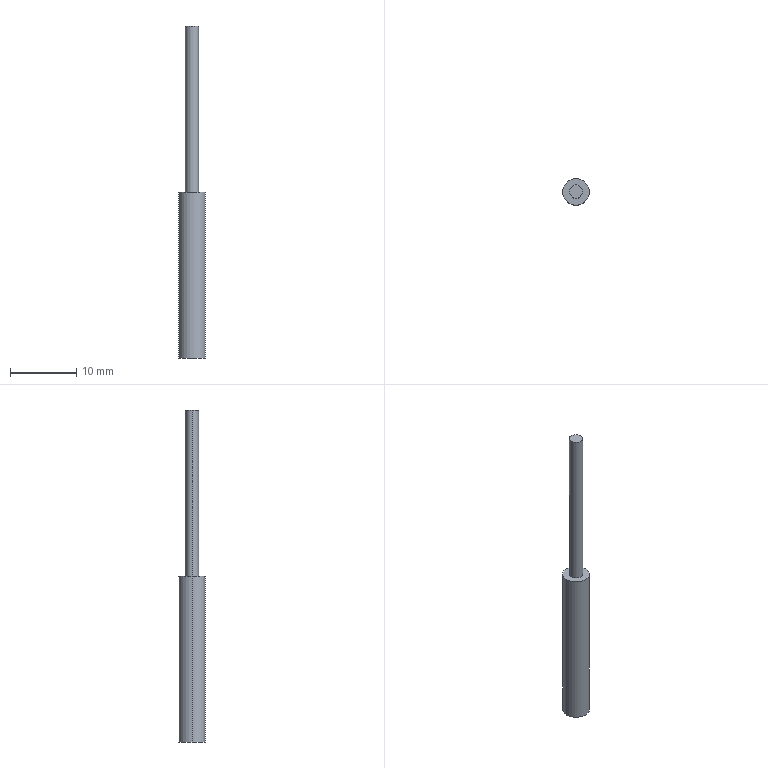Part | STEP file | e2e-cr8 | 1 solid | 7 faces | box 4 x 4 x 50 mm | volume 392.699 mm3 | cylinder 4 | plane 3 | commonest cylinder face diameters 2 x2 4 x2
STEP:
#1=CARTESIAN_POINT('',(1.,0.,50.));
#2=VERTEX_POINT('',#1);
#3=CARTESIAN_POINT('',(-1.,0.,50.));
#4=VERTEX_POINT('',#3);
#5=CARTESIAN_POINT('',(0.,0.,50.));
#6=DIRECTION('',(0.,0.,1.));
#7=DIRECTION('',(1.,0.,0.));
#8=AXIS2_PLACEMENT_3D('',#5,#6,#7);
#9=CIRCLE('',#8,1.);
#10=EDGE_CURVE('',#2,#4,#9,.T.);
#11=ORIENTED_EDGE('',*,*,#10,.F.);
#12=CARTESIAN_POINT('',(1.,0.,25.));
#13=VERTEX_POINT('',#12);
#14=CARTESIAN_POINT('',(1.,0.,50.));
#15=DIRECTION('',(0.,0.,-1.));
#16=VECTOR('',#15,1000.);
#17=LINE('',#14,#16);
#18=EDGE_CURVE('',#2,#13,#17,.T.);
#19=ORIENTED_EDGE('',*,*,#18,.T.);
#20=CARTESIAN_POINT('',(-1.,0.,25.));
#21=VERTEX_POINT('',#20);
#22=CARTESIAN_POINT('',(0.,0.,25.));
#23=DIRECTION('',(0.,0.,1.));
#24=DIRECTION('',(1.,0.,0.));
#25=AXIS2_PLACEMENT_3D('',#22,#23,#24);
#26=CIRCLE('',#25,1.);
#27=EDGE_CURVE('',#13,#21,#26,.T.);
#28=ORIENTED_EDGE('',*,*,#27,.T.);
#29=CARTESIAN_POINT('',(-1.,0.,50.));
#30=DIRECTION('',(0.,0.,-1.));
#31=VECTOR('',#30,1000.);
#32=LINE('',#29,#31);
#33=EDGE_CURVE('',#4,#21,#32,.T.);
#34=ORIENTED_EDGE('',*,*,#33,.F.);
#35=EDGE_LOOP('',(#11,#19,#28,#34));
#36=FACE_OUTER_BOUND('',#35,.T.);
#37=CARTESIAN_POINT('',(0.,0.,50.));
#38=DIRECTION('',(0.,0.,-1.));
#39=DIRECTION('',(-1.,0.,0.));
#40=AXIS2_PLACEMENT_3D('',#37,#38,#39);
#41=CYLINDRICAL_SURFACE('',#40,1.);
#42=ADVANCED_FACE('',(#36),#41,.T.);
#43=CARTESIAN_POINT('',(2.,0.,25.));
#44=VERTEX_POINT('',#43);
#45=CARTESIAN_POINT('',(-2.,0.,25.));
#46=VERTEX_POINT('',#45);
#47=CARTESIAN_POINT('',(0.,0.,25.));
#48=DIRECTION('',(0.,0.,1.));
#49=DIRECTION('',(1.,0.,0.));
#50=AXIS2_PLACEMENT_3D('',#47,#48,#49);
#51=CIRCLE('',#50,2.);
#52=EDGE_CURVE('',#44,#46,#51,.T.);
#53=ORIENTED_EDGE('',*,*,#52,.F.);
#54=CARTESIAN_POINT('',(2.,0.,0.));
#55=VERTEX_POINT('',#54);
#56=CARTESIAN_POINT('',(2.,0.,25.));
#57=DIRECTION('',(0.,0.,-1.));
#58=VECTOR('',#57,1000.);
#59=LINE('',#56,#58);
#60=EDGE_CURVE('',#44,#55,#59,.T.);
#61=ORIENTED_EDGE('',*,*,#60,.T.);
#62=CARTESIAN_POINT('',(-2.,0.,0.));
#63=VERTEX_POINT('',#62);
#64=CARTESIAN_POINT('',(0.,0.,0.));
#65=DIRECTION('',(0.,0.,1.));
#66=DIRECTION('',(1.,0.,0.));
#67=AXIS2_PLACEMENT_3D('',#64,#65,#66);
#68=CIRCLE('',#67,2.);
#69=EDGE_CURVE('',#55,#63,#68,.T.);
#70=ORIENTED_EDGE('',*,*,#69,.T.);
#71=CARTESIAN_POINT('',(-2.,0.,25.));
#72=DIRECTION('',(0.,0.,-1.));
#73=VECTOR('',#72,1000.);
#74=LINE('',#71,#73);
#75=EDGE_CURVE('',#46,#63,#74,.T.);
#76=ORIENTED_EDGE('',*,*,#75,.F.);
#77=EDGE_LOOP('',(#53,#61,#70,#76));
#78=FACE_OUTER_BOUND('',#77,.T.);
#79=CARTESIAN_POINT('',(0.,0.,25.));
#80=DIRECTION('',(0.,0.,-1.));
#81=DIRECTION('',(-1.,0.,0.));
#82=AXIS2_PLACEMENT_3D('',#79,#80,#81);
#83=CYLINDRICAL_SURFACE('',#82,2.);
#84=ADVANCED_FACE('',(#78),#83,.T.);
#85=CARTESIAN_POINT('',(0.,0.,25.));
#86=DIRECTION('',(0.,0.,1.));
#87=DIRECTION('',(1.,0.,0.));
#88=AXIS2_PLACEMENT_3D('',#85,#86,#87);
#89=CIRCLE('',#88,2.);
#90=EDGE_CURVE('',#46,#44,#89,.T.);
#91=ORIENTED_EDGE('',*,*,#90,.T.);
#92=ORIENTED_EDGE('',*,*,#52,.T.);
#93=EDGE_LOOP('',(#91,#92));
#94=FACE_OUTER_BOUND('',#93,.T.);
#95=CARTESIAN_POINT('',(0.,0.,25.));
#96=DIRECTION('',(0.,0.,1.));
#97=DIRECTION('',(1.,0.,0.));
#98=AXIS2_PLACEMENT_3D('',#95,#96,#97);
#99=CIRCLE('',#98,1.);
#100=EDGE_CURVE('',#21,#13,#99,.T.);
#101=ORIENTED_EDGE('',*,*,#100,.F.);
#102=ORIENTED_EDGE('',*,*,#27,.F.);
#103=EDGE_LOOP('',(#101,#102));
#104=FACE_BOUND('',#103,.T.);
#105=CARTESIAN_POINT('',(0.,0.,25.));
#106=DIRECTION('',(0.,0.,1.));
#107=DIRECTION('',(1.,0.,0.));
#108=AXIS2_PLACEMENT_3D('',#105,#106,#107);
#109=PLANE('',#108);
#110=ADVANCED_FACE('',(#94,#104),#109,.T.);
#111=ORIENTED_EDGE('',*,*,#60,.F.);
#112=ORIENTED_EDGE('',*,*,#90,.F.);
#113=ORIENTED_EDGE('',*,*,#75,.T.);
#114=CARTESIAN_POINT('',(0.,0.,0.));
#115=DIRECTION('',(0.,0.,1.));
#116=DIRECTION('',(1.,0.,0.));
#117=AXIS2_PLACEMENT_3D('',#114,#115,#116);
#118=CIRCLE('',#117,2.);
#119=EDGE_CURVE('',#63,#55,#118,.T.);
#120=ORIENTED_EDGE('',*,*,#119,.T.);
#121=EDGE_LOOP('',(#111,#112,#113,#120));
#122=FACE_OUTER_BOUND('',#121,.T.);
#123=CARTESIAN_POINT('',(0.,0.,25.));
#124=DIRECTION('',(0.,0.,-1.));
#125=DIRECTION('',(-1.,0.,0.));
#126=AXIS2_PLACEMENT_3D('',#123,#124,#125);
#127=CYLINDRICAL_SURFACE('',#126,2.);
#128=ADVANCED_FACE('',(#122),#127,.T.);
#129=ORIENTED_EDGE('',*,*,#119,.F.);
#130=ORIENTED_EDGE('',*,*,#69,.F.);
#131=EDGE_LOOP('',(#129,#130));
#132=FACE_OUTER_BOUND('',#131,.T.);
#133=CARTESIAN_POINT('',(0.,0.,0.));
#134=DIRECTION('',(0.,0.,1.));
#135=DIRECTION('',(1.,0.,0.));
#136=AXIS2_PLACEMENT_3D('',#133,#134,#135);
#137=PLANE('',#136);
#138=ADVANCED_FACE('',(#132),#137,.F.);
#139=ORIENTED_EDGE('',*,*,#18,.F.);
#140=CARTESIAN_POINT('',(0.,0.,50.));
#141=DIRECTION('',(0.,0.,1.));
#142=DIRECTION('',(1.,0.,0.));
#143=AXIS2_PLACEMENT_3D('',#140,#141,#142);
#144=CIRCLE('',#143,1.);
#145=EDGE_CURVE('',#4,#2,#144,.T.);
#146=ORIENTED_EDGE('',*,*,#145,.F.);
#147=ORIENTED_EDGE('',*,*,#33,.T.);
#148=ORIENTED_EDGE('',*,*,#100,.T.);
#149=EDGE_LOOP('',(#139,#146,#147,#148));
#150=FACE_OUTER_BOUND('',#149,.T.);
#151=CARTESIAN_POINT('',(0.,0.,50.));
#152=DIRECTION('',(0.,0.,-1.));
#153=DIRECTION('',(-1.,0.,0.));
#154=AXIS2_PLACEMENT_3D('',#151,#152,#153);
#155=CYLINDRICAL_SURFACE('',#154,1.);
#156=ADVANCED_FACE('',(#150),#155,.T.);
#157=ORIENTED_EDGE('',*,*,#145,.T.);
#158=ORIENTED_EDGE('',*,*,#10,.T.);
#159=EDGE_LOOP('',(#157,#158));
#160=FACE_OUTER_BOUND('',#159,.T.);
#161=CARTESIAN_POINT('',(0.,0.,50.));
#162=DIRECTION('',(0.,0.,1.));
#163=DIRECTION('',(1.,0.,0.));
#164=AXIS2_PLACEMENT_3D('',#161,#162,#163);
#165=PLANE('',#164);
#166=ADVANCED_FACE('',(#160),#165,.T.);
#167=CLOSED_SHELL('',(#42,#84,#110,#128,#138,#156,#166));
#168=MANIFOLD_SOLID_BREP('',#167);
#169=CARTESIAN_POINT('',(0.,0.,0.));
#170=DIRECTION('',(0.,0.,1.));
#171=DIRECTION('',(1.,0.,0.));
#172=AXIS2_PLACEMENT_3D('',#169,#170,#171);
#173=(LENGTH_UNIT()NAMED_UNIT(*)SI_UNIT(.MILLI.,.METRE.));
#174=UNCERTAINTY_MEASURE_WITH_UNIT(LENGTH_MEASURE(0.00001),#173,'','');
#175=(NAMED_UNIT(*)PLANE_ANGLE_UNIT()SI_UNIT($,.RADIAN.));
#176=(NAMED_UNIT(*)SI_UNIT($,.STERADIAN.)SOLID_ANGLE_UNIT());
#177=(GEOMETRIC_REPRESENTATION_CONTEXT(3)GLOBAL_UNCERTAINTY_ASSIGNED_CONTEXT((#174))GLOBAL_UNIT_ASSIGNED_CONTEXT((#173,#175,#176))REPRESENTATION_CONTEXT('',''));
#178=ADVANCED_BREP_SHAPE_REPRESENTATION('',(#168,#172),#177);